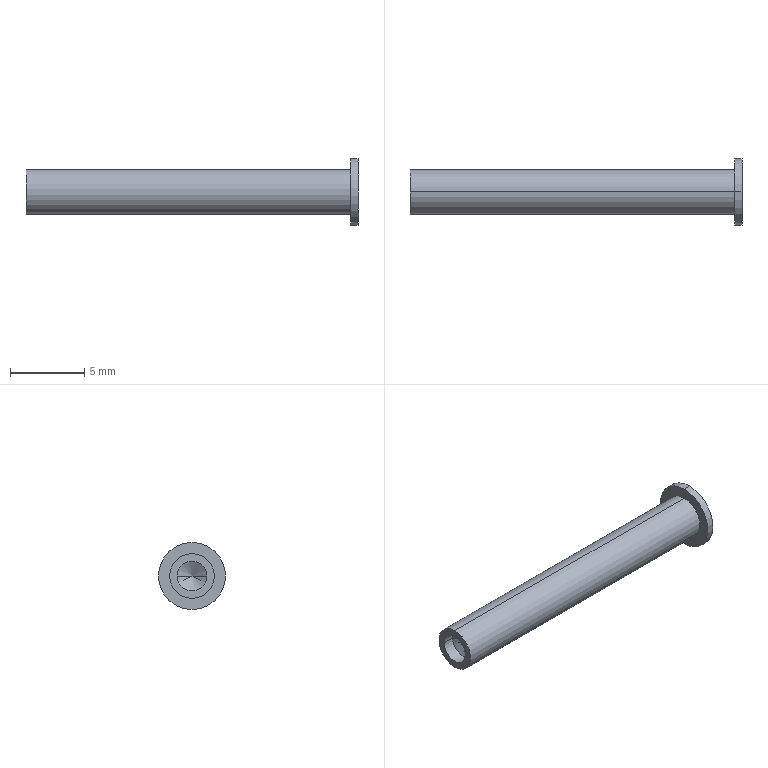Part | STEP file | _X2_751F4E45_X0_MS731-1_X2_8_11 | 1 solid | 11 faces | box 22.3 x 4.5 x 4.5 mm | volume 158.929 mm3 | cylinder 6 | plane 3 | cone 2 | commonest cylinder face diameters 2 x2 3 x2 4.5 x2
STEP:
#1=CARTESIAN_POINT('',(0.,0.,0.));
#2=DIRECTION('',(0.,0.,1.));
#3=DIRECTION('',(1.,0.,0.));
#4=AXIS2_PLACEMENT_3D('',#1,#2,#3);
#5=CARTESIAN_POINT('',(26.2,21.281,-110.75));
#6=VERTEX_POINT('',#5);
#7=CARTESIAN_POINT('',(26.2,21.281,-106.25));
#8=VERTEX_POINT('',#7);
#9=CARTESIAN_POINT('',(26.2,21.281,-108.5));
#10=DIRECTION('',(-1.,0.,0.));
#11=DIRECTION('',(0.,0.,-1.));
#12=AXIS2_PLACEMENT_3D('',#9,#10,#11);
#13=CIRCLE('',#12,2.25);
#14=CARTESIAN_POINT('',(26.2,21.281,-108.5));
#15=DIRECTION('',(-1.,0.,0.));
#16=DIRECTION('',(0.,0.,1.));
#17=AXIS2_PLACEMENT_3D('',#14,#15,#16);
#18=PLANE('',#17);
#19=CARTESIAN_POINT('',(0.,0.));
#20=DIRECTION('',(-1.,0.));
#21=AXIS2_PLACEMENT_2D('',#19,#20);
#22=CIRCLE('',#21,2.25);
#23=(GEOMETRIC_REPRESENTATION_CONTEXT(2)PARAMETRIC_REPRESENTATION_CONTEXT()REPRESENTATION_CONTEXT('',''));
#24=DEFINITIONAL_REPRESENTATION('',(#22),#23);
#25=PCURVE('',#18,#24);
#26=CARTESIAN_POINT('',(27.815,21.281,-108.5));
#27=DIRECTION('',(-1.,0.,0.));
#28=DIRECTION('',(0.,0.,1.));
#29=AXIS2_PLACEMENT_3D('',#26,#27,#28);
#30=CYLINDRICAL_SURFACE('',#29,2.25);
#31=CARTESIAN_POINT('',(3.142,1.615));
#32=DIRECTION('',(1.,0.));
#33=VECTOR('',#32,1.);
#34=LINE('',#31,#33);
#35=(GEOMETRIC_REPRESENTATION_CONTEXT(2)PARAMETRIC_REPRESENTATION_CONTEXT()REPRESENTATION_CONTEXT('',''));
#36=DEFINITIONAL_REPRESENTATION('',(#34),#35);
#37=PCURVE('',#30,#36);
#38=SURFACE_CURVE('',#13,(#25,#37),.PCURVE_S1.);
#39=EDGE_CURVE('',#6,#8,#38,.T.);
#40=ORIENTED_EDGE('',*,*,#39,.F.);
#41=CARTESIAN_POINT('',(26.2,21.281,-108.5));
#42=DIRECTION('',(-1.,0.,0.));
#43=DIRECTION('',(0.,0.,1.));
#44=AXIS2_PLACEMENT_3D('',#41,#42,#43);
#45=CIRCLE('',#44,2.25);
#46=CARTESIAN_POINT('',(0.,0.));
#47=DIRECTION('',(1.,0.));
#48=AXIS2_PLACEMENT_2D('',#46,#47);
#49=CIRCLE('',#48,2.25);
#50=(GEOMETRIC_REPRESENTATION_CONTEXT(2)PARAMETRIC_REPRESENTATION_CONTEXT()REPRESENTATION_CONTEXT('',''));
#51=DEFINITIONAL_REPRESENTATION('',(#49),#50);
#52=PCURVE('',#18,#51);
#53=CARTESIAN_POINT('',(27.815,21.281,-108.5));
#54=DIRECTION('',(-1.,0.,0.));
#55=DIRECTION('',(0.,0.,1.));
#56=AXIS2_PLACEMENT_3D('',#53,#54,#55);
#57=CYLINDRICAL_SURFACE('',#56,2.25);
#58=CARTESIAN_POINT('',(0.,1.615));
#59=DIRECTION('',(1.,0.));
#60=VECTOR('',#59,1.);
#61=LINE('',#58,#60);
#62=(GEOMETRIC_REPRESENTATION_CONTEXT(2)PARAMETRIC_REPRESENTATION_CONTEXT()REPRESENTATION_CONTEXT('',''));
#63=DEFINITIONAL_REPRESENTATION('',(#61),#62);
#64=PCURVE('',#57,#63);
#65=SURFACE_CURVE('',#45,(#52,#64),.PCURVE_S1.);
#66=EDGE_CURVE('',#8,#6,#65,.T.);
#67=ORIENTED_EDGE('',*,*,#66,.F.);
#68=EDGE_LOOP('',(#40,#67));
#69=FACE_BOUND('',#68,.F.);
#70=CARTESIAN_POINT('',(26.2,21.281,-110.));
#71=VERTEX_POINT('',#70);
#72=CARTESIAN_POINT('',(26.2,21.281,-107.));
#73=VERTEX_POINT('',#72);
#74=CARTESIAN_POINT('',(26.2,21.281,-108.5));
#75=DIRECTION('',(1.,0.,0.));
#76=DIRECTION('',(0.,0.,-1.));
#77=AXIS2_PLACEMENT_3D('',#74,#75,#76);
#78=CIRCLE('',#77,1.5);
#79=CARTESIAN_POINT('',(-1.5,0.));
#80=CARTESIAN_POINT('',(-1.5,2.598));
#81=CARTESIAN_POINT('',(0.75,1.299));
#82=CARTESIAN_POINT('',(3.,0.));
#83=CARTESIAN_POINT('',(0.75,-1.299));
#84=CARTESIAN_POINT('',(-1.5,-2.598));
#85=CARTESIAN_POINT('',(-1.5,0.));
#86=(BOUNDED_CURVE()B_SPLINE_CURVE(2,(#79,#80,#81,#82,#83,#84,#85),.UNSPECIFIED.,.T.,.F.)B_SPLINE_CURVE_WITH_KNOTS((1,2,2,2,2,1),(-2.094,0.,2.094,4.189,6.283,8.378),.UNSPECIFIED.)CURVE()GEOMETRIC_REPRESENTATION_ITEM()RATIONAL_B_SPLINE_CURVE((1.,0.5,1.,0.5,1.,0.5,1.))REPRESENTATION_ITEM(''));
#87=(GEOMETRIC_REPRESENTATION_CONTEXT(2)PARAMETRIC_REPRESENTATION_CONTEXT()REPRESENTATION_CONTEXT('',''));
#88=DEFINITIONAL_REPRESENTATION('',(#86),#87);
#89=PCURVE('',#18,#88);
#90=CARTESIAN_POINT('',(27.815,21.281,-108.5));
#91=DIRECTION('',(-1.,0.,0.));
#92=DIRECTION('',(0.,0.,1.));
#93=AXIS2_PLACEMENT_3D('',#90,#91,#92);
#94=CYLINDRICAL_SURFACE('',#93,1.5);
#95=CARTESIAN_POINT('',(3.142,1.615));
#96=DIRECTION('',(-1.,0.));
#97=VECTOR('',#96,1.);
#98=LINE('',#95,#97);
#99=(GEOMETRIC_REPRESENTATION_CONTEXT(2)PARAMETRIC_REPRESENTATION_CONTEXT()REPRESENTATION_CONTEXT('',''));
#100=DEFINITIONAL_REPRESENTATION('',(#98),#99);
#101=PCURVE('',#94,#100);
#102=SURFACE_CURVE('',#78,(#89,#101),.PCURVE_S1.);
#103=EDGE_CURVE('',#71,#73,#102,.T.);
#104=ORIENTED_EDGE('',*,*,#103,.F.);
#105=CARTESIAN_POINT('',(26.2,21.281,-108.5));
#106=DIRECTION('',(1.,0.,0.));
#107=DIRECTION('',(0.,0.,1.));
#108=AXIS2_PLACEMENT_3D('',#105,#106,#107);
#109=CIRCLE('',#108,1.5);
#110=CARTESIAN_POINT('',(1.5,0.));
#111=CARTESIAN_POINT('',(1.5,-2.598));
#112=CARTESIAN_POINT('',(-0.75,-1.299));
#113=CARTESIAN_POINT('',(-3.,0.));
#114=CARTESIAN_POINT('',(-0.75,1.299));
#115=CARTESIAN_POINT('',(1.5,2.598));
#116=CARTESIAN_POINT('',(1.5,0.));
#117=(BOUNDED_CURVE()B_SPLINE_CURVE(2,(#110,#111,#112,#113,#114,#115,#116),.UNSPECIFIED.,.T.,.F.)B_SPLINE_CURVE_WITH_KNOTS((1,2,2,2,2,1),(-2.094,0.,2.094,4.189,6.283,8.378),.UNSPECIFIED.)CURVE()GEOMETRIC_REPRESENTATION_ITEM()RATIONAL_B_SPLINE_CURVE((1.,0.5,1.,0.5,1.,0.5,1.))REPRESENTATION_ITEM(''));
#118=(GEOMETRIC_REPRESENTATION_CONTEXT(2)PARAMETRIC_REPRESENTATION_CONTEXT()REPRESENTATION_CONTEXT('',''));
#119=DEFINITIONAL_REPRESENTATION('',(#117),#118);
#120=PCURVE('',#18,#119);
#121=CARTESIAN_POINT('',(27.815,21.281,-108.5));
#122=DIRECTION('',(-1.,0.,0.));
#123=DIRECTION('',(0.,0.,1.));
#124=AXIS2_PLACEMENT_3D('',#121,#122,#123);
#125=CYLINDRICAL_SURFACE('',#124,1.5);
#126=CARTESIAN_POINT('',(6.283,1.615));
#127=DIRECTION('',(-1.,0.));
#128=VECTOR('',#127,1.);
#129=LINE('',#126,#128);
#130=(GEOMETRIC_REPRESENTATION_CONTEXT(2)PARAMETRIC_REPRESENTATION_CONTEXT()REPRESENTATION_CONTEXT('',''));
#131=DEFINITIONAL_REPRESENTATION('',(#129),#130);
#132=PCURVE('',#125,#131);
#133=SURFACE_CURVE('',#109,(#120,#132),.PCURVE_S1.);
#134=EDGE_CURVE('',#73,#71,#133,.T.);
#135=ORIENTED_EDGE('',*,*,#134,.F.);
#136=EDGE_LOOP('',(#104,#135));
#137=FACE_BOUND('',#136,.F.);
#138=ADVANCED_FACE('',(#69,#137),#18,.T.);
#139=CARTESIAN_POINT('',(26.7,21.281,-110.75));
#140=VERTEX_POINT('',#139);
#141=CARTESIAN_POINT('',(26.2,21.281,-110.75));
#142=DIRECTION('',(1.,0.,0.));
#143=VECTOR('',#142,1.);
#144=LINE('',#141,#143);
#145=CARTESIAN_POINT('',(3.142,1.615));
#146=DIRECTION('',(0.,-1.));
#147=VECTOR('',#146,1.);
#148=LINE('',#145,#147);
#149=(GEOMETRIC_REPRESENTATION_CONTEXT(2)PARAMETRIC_REPRESENTATION_CONTEXT()REPRESENTATION_CONTEXT('',''));
#150=DEFINITIONAL_REPRESENTATION('',(#148),#149);
#151=PCURVE('',#30,#150);
#152=CARTESIAN_POINT('',(3.142,1.615));
#153=DIRECTION('',(0.,-1.));
#154=VECTOR('',#153,1.);
#155=LINE('',#152,#154);
#156=(GEOMETRIC_REPRESENTATION_CONTEXT(2)PARAMETRIC_REPRESENTATION_CONTEXT()REPRESENTATION_CONTEXT('',''));
#157=DEFINITIONAL_REPRESENTATION('',(#155),#156);
#158=PCURVE('',#57,#157);
#159=SURFACE_CURVE('',#144,(#151,#158),.PCURVE_S1.);
#160=EDGE_CURVE('',#6,#140,#159,.T.);
#161=ORIENTED_EDGE('',*,*,#160,.T.);
#162=CARTESIAN_POINT('',(26.7,21.281,-106.25));
#163=VERTEX_POINT('',#162);
#164=CARTESIAN_POINT('',(26.7,21.281,-108.5));
#165=DIRECTION('',(1.,0.,0.));
#166=DIRECTION('',(0.,0.,1.));
#167=AXIS2_PLACEMENT_3D('',#164,#165,#166);
#168=CIRCLE('',#167,2.25);
#169=CARTESIAN_POINT('',(6.283,1.115));
#170=DIRECTION('',(-1.,0.));
#171=VECTOR('',#170,1.);
#172=LINE('',#169,#171);
#173=(GEOMETRIC_REPRESENTATION_CONTEXT(2)PARAMETRIC_REPRESENTATION_CONTEXT()REPRESENTATION_CONTEXT('',''));
#174=DEFINITIONAL_REPRESENTATION('',(#172),#173);
#175=PCURVE('',#30,#174);
#176=CARTESIAN_POINT('',(26.7,21.281,-108.5));
#177=DIRECTION('',(-1.,0.,0.));
#178=DIRECTION('',(0.,0.,1.));
#179=AXIS2_PLACEMENT_3D('',#176,#177,#178);
#180=PLANE('',#179);
#181=CARTESIAN_POINT('',(2.25,0.));
#182=CARTESIAN_POINT('',(2.25,-3.897));
#183=CARTESIAN_POINT('',(-1.125,-1.949));
#184=CARTESIAN_POINT('',(-4.5,0.));
#185=CARTESIAN_POINT('',(-1.125,1.949));
#186=CARTESIAN_POINT('',(2.25,3.897));
#187=CARTESIAN_POINT('',(2.25,0.));
#188=(BOUNDED_CURVE()B_SPLINE_CURVE(2,(#181,#182,#183,#184,#185,#186,#187),.UNSPECIFIED.,.T.,.F.)B_SPLINE_CURVE_WITH_KNOTS((1,2,2,2,2,1),(-2.094,0.,2.094,4.189,6.283,8.378),.UNSPECIFIED.)CURVE()GEOMETRIC_REPRESENTATION_ITEM()RATIONAL_B_SPLINE_CURVE((1.,0.5,1.,0.5,1.,0.5,1.))REPRESENTATION_ITEM(''));
#189=(GEOMETRIC_REPRESENTATION_CONTEXT(2)PARAMETRIC_REPRESENTATION_CONTEXT()REPRESENTATION_CONTEXT('',''));
#190=DEFINITIONAL_REPRESENTATION('',(#188),#189);
#191=PCURVE('',#180,#190);
#192=SURFACE_CURVE('',#168,(#175,#191),.PCURVE_S1.);
#193=EDGE_CURVE('',#163,#140,#192,.T.);
#194=ORIENTED_EDGE('',*,*,#193,.F.);
#195=CARTESIAN_POINT('',(26.2,21.281,-106.25));
#196=DIRECTION('',(1.,0.,0.));
#197=VECTOR('',#196,1.);
#198=LINE('',#195,#197);
#199=CARTESIAN_POINT('',(6.283,1.615));
#200=DIRECTION('',(0.,-1.));
#201=VECTOR('',#200,1.);
#202=LINE('',#199,#201);
#203=(GEOMETRIC_REPRESENTATION_CONTEXT(2)PARAMETRIC_REPRESENTATION_CONTEXT()REPRESENTATION_CONTEXT('',''));
#204=DEFINITIONAL_REPRESENTATION('',(#202),#203);
#205=PCURVE('',#30,#204);
#206=CARTESIAN_POINT('',(0.,1.615));
#207=DIRECTION('',(0.,-1.));
#208=VECTOR('',#207,1.);
#209=LINE('',#206,#208);
#210=(GEOMETRIC_REPRESENTATION_CONTEXT(2)PARAMETRIC_REPRESENTATION_CONTEXT()REPRESENTATION_CONTEXT('',''));
#211=DEFINITIONAL_REPRESENTATION('',(#209),#210);
#212=PCURVE('',#57,#211);
#213=SURFACE_CURVE('',#198,(#205,#212),.PCURVE_S1.);
#214=EDGE_CURVE('',#8,#163,#213,.T.);
#215=ORIENTED_EDGE('',*,*,#214,.F.);
#216=ORIENTED_EDGE('',*,*,#39,.F.);
#217=EDGE_LOOP('',(#161,#194,#215,#216));
#218=FACE_BOUND('',#217,.T.);
#219=ADVANCED_FACE('',(#218),#30,.T.);
#220=ORIENTED_EDGE('',*,*,#160,.F.);
#221=ORIENTED_EDGE('',*,*,#66,.F.);
#222=ORIENTED_EDGE('',*,*,#214,.T.);
#223=CARTESIAN_POINT('',(26.7,21.281,-108.5));
#224=DIRECTION('',(1.,0.,0.));
#225=DIRECTION('',(0.,0.,-1.));
#226=AXIS2_PLACEMENT_3D('',#223,#224,#225);
#227=CIRCLE('',#226,2.25);
#228=CARTESIAN_POINT('',(3.142,1.115));
#229=DIRECTION('',(-1.,0.));
#230=VECTOR('',#229,1.);
#231=LINE('',#228,#230);
#232=(GEOMETRIC_REPRESENTATION_CONTEXT(2)PARAMETRIC_REPRESENTATION_CONTEXT()REPRESENTATION_CONTEXT('',''));
#233=DEFINITIONAL_REPRESENTATION('',(#231),#232);
#234=PCURVE('',#57,#233);
#235=CARTESIAN_POINT('',(-2.25,0.));
#236=CARTESIAN_POINT('',(-2.25,3.897));
#237=CARTESIAN_POINT('',(1.125,1.949));
#238=CARTESIAN_POINT('',(4.5,0.));
#239=CARTESIAN_POINT('',(1.125,-1.949));
#240=CARTESIAN_POINT('',(-2.25,-3.897));
#241=CARTESIAN_POINT('',(-2.25,0.));
#242=(BOUNDED_CURVE()B_SPLINE_CURVE(2,(#235,#236,#237,#238,#239,#240,#241),.UNSPECIFIED.,.T.,.F.)B_SPLINE_CURVE_WITH_KNOTS((1,2,2,2,2,1),(-2.094,0.,2.094,4.189,6.283,8.378),.UNSPECIFIED.)CURVE()GEOMETRIC_REPRESENTATION_ITEM()RATIONAL_B_SPLINE_CURVE((1.,0.5,1.,0.5,1.,0.5,1.))REPRESENTATION_ITEM(''));
#243=(GEOMETRIC_REPRESENTATION_CONTEXT(2)PARAMETRIC_REPRESENTATION_CONTEXT()REPRESENTATION_CONTEXT('',''));
#244=DEFINITIONAL_REPRESENTATION('',(#242),#243);
#245=PCURVE('',#180,#244);
#246=SURFACE_CURVE('',#227,(#234,#245),.PCURVE_S1.);
#247=EDGE_CURVE('',#140,#163,#246,.T.);
#248=ORIENTED_EDGE('',*,*,#247,.F.);
#249=EDGE_LOOP('',(#220,#221,#222,#248));
#250=FACE_BOUND('',#249,.T.);
#251=ADVANCED_FACE('',(#250),#57,.T.);
#252=ORIENTED_EDGE('',*,*,#247,.F.);
#253=ORIENTED_EDGE('',*,*,#193,.F.);
#254=EDGE_LOOP('',(#252,#253));
#255=FACE_BOUND('',#254,.F.);
#256=ADVANCED_FACE('',(#255),#180,.F.);
#257=CARTESIAN_POINT('',(4.4,21.281,-110.));
#258=VERTEX_POINT('',#257);
#259=CARTESIAN_POINT('',(4.4,21.281,-110.));
#260=DIRECTION('',(1.,0.,0.));
#261=VECTOR('',#260,1.);
#262=LINE('',#259,#261);
#263=CARTESIAN_POINT('',(3.142,23.415));
#264=DIRECTION('',(0.,-1.));
#265=VECTOR('',#264,1.);
#266=LINE('',#263,#265);
#267=(GEOMETRIC_REPRESENTATION_CONTEXT(2)PARAMETRIC_REPRESENTATION_CONTEXT()REPRESENTATION_CONTEXT('',''));
#268=DEFINITIONAL_REPRESENTATION('',(#266),#267);
#269=PCURVE('',#94,#268);
#270=CARTESIAN_POINT('',(3.142,23.415));
#271=DIRECTION('',(0.,-1.));
#272=VECTOR('',#271,1.);
#273=LINE('',#270,#272);
#274=(GEOMETRIC_REPRESENTATION_CONTEXT(2)PARAMETRIC_REPRESENTATION_CONTEXT()REPRESENTATION_CONTEXT('',''));
#275=DEFINITIONAL_REPRESENTATION('',(#273),#274);
#276=PCURVE('',#125,#275);
#277=SURFACE_CURVE('',#262,(#269,#276),.PCURVE_S1.);
#278=EDGE_CURVE('',#258,#71,#277,.T.);
#279=ORIENTED_EDGE('',*,*,#278,.F.);
#280=CARTESIAN_POINT('',(4.4,21.281,-107.));
#281=VERTEX_POINT('',#280);
#282=CARTESIAN_POINT('',(4.4,21.281,-108.5));
#283=DIRECTION('',(-1.,0.,0.));
#284=DIRECTION('',(0.,0.,1.));
#285=AXIS2_PLACEMENT_3D('',#282,#283,#284);
#286=CIRCLE('',#285,1.5);
#287=CARTESIAN_POINT('',(0.,23.415));
#288=DIRECTION('',(1.,0.));
#289=VECTOR('',#288,1.);
#290=LINE('',#287,#289);
#291=(GEOMETRIC_REPRESENTATION_CONTEXT(2)PARAMETRIC_REPRESENTATION_CONTEXT()REPRESENTATION_CONTEXT('',''));
#292=DEFINITIONAL_REPRESENTATION('',(#290),#291);
#293=PCURVE('',#94,#292);
#294=CARTESIAN_POINT('',(4.4,21.281,-108.5));
#295=DIRECTION('',(-1.,0.,0.));
#296=DIRECTION('',(0.,0.,1.));
#297=AXIS2_PLACEMENT_3D('',#294,#295,#296);
#298=PLANE('',#297);
#299=CARTESIAN_POINT('',(0.,0.));
#300=DIRECTION('',(1.,0.));
#301=AXIS2_PLACEMENT_2D('',#299,#300);
#302=CIRCLE('',#301,1.5);
#303=(GEOMETRIC_REPRESENTATION_CONTEXT(2)PARAMETRIC_REPRESENTATION_CONTEXT()REPRESENTATION_CONTEXT('',''));
#304=DEFINITIONAL_REPRESENTATION('',(#302),#303);
#305=PCURVE('',#298,#304);
#306=SURFACE_CURVE('',#286,(#293,#305),.PCURVE_S1.);
#307=EDGE_CURVE('',#281,#258,#306,.T.);
#308=ORIENTED_EDGE('',*,*,#307,.F.);
#309=CARTESIAN_POINT('',(4.4,21.281,-107.));
#310=DIRECTION('',(1.,0.,0.));
#311=VECTOR('',#310,1.);
#312=LINE('',#309,#311);
#313=CARTESIAN_POINT('',(0.,23.415));
#314=DIRECTION('',(0.,-1.));
#315=VECTOR('',#314,1.);
#316=LINE('',#313,#315);
#317=(GEOMETRIC_REPRESENTATION_CONTEXT(2)PARAMETRIC_REPRESENTATION_CONTEXT()REPRESENTATION_CONTEXT('',''));
#318=DEFINITIONAL_REPRESENTATION('',(#316),#317);
#319=PCURVE('',#94,#318);
#320=CARTESIAN_POINT('',(6.283,23.415));
#321=DIRECTION('',(0.,-1.));
#322=VECTOR('',#321,1.);
#323=LINE('',#320,#322);
#324=(GEOMETRIC_REPRESENTATION_CONTEXT(2)PARAMETRIC_REPRESENTATION_CONTEXT()REPRESENTATION_CONTEXT('',''));
#325=DEFINITIONAL_REPRESENTATION('',(#323),#324);
#326=PCURVE('',#125,#325);
#327=SURFACE_CURVE('',#312,(#319,#326),.PCURVE_S1.);
#328=EDGE_CURVE('',#281,#73,#327,.T.);
#329=ORIENTED_EDGE('',*,*,#328,.T.);
#330=ORIENTED_EDGE('',*,*,#103,.F.);
#331=EDGE_LOOP('',(#279,#308,#329,#330));
#332=FACE_BOUND('',#331,.T.);
#333=ADVANCED_FACE('',(#332),#94,.T.);
#334=ORIENTED_EDGE('',*,*,#278,.T.);
#335=ORIENTED_EDGE('',*,*,#134,.F.);
#336=ORIENTED_EDGE('',*,*,#328,.F.);
#337=CARTESIAN_POINT('',(4.4,21.281,-108.5));
#338=DIRECTION('',(-1.,0.,0.));
#339=DIRECTION('',(0.,0.,-1.));
#340=AXIS2_PLACEMENT_3D('',#337,#338,#339);
#341=CIRCLE('',#340,1.5);
#342=CARTESIAN_POINT('',(3.142,23.415));
#343=DIRECTION('',(1.,0.));
#344=VECTOR('',#343,1.);
#345=LINE('',#342,#344);
#346=(GEOMETRIC_REPRESENTATION_CONTEXT(2)PARAMETRIC_REPRESENTATION_CONTEXT()REPRESENTATION_CONTEXT('',''));
#347=DEFINITIONAL_REPRESENTATION('',(#345),#346);
#348=PCURVE('',#125,#347);
#349=CARTESIAN_POINT('',(0.,0.));
#350=DIRECTION('',(-1.,0.));
#351=AXIS2_PLACEMENT_2D('',#349,#350);
#352=CIRCLE('',#351,1.5);
#353=(GEOMETRIC_REPRESENTATION_CONTEXT(2)PARAMETRIC_REPRESENTATION_CONTEXT()REPRESENTATION_CONTEXT('',''));
#354=DEFINITIONAL_REPRESENTATION('',(#352),#353);
#355=PCURVE('',#298,#354);
#356=SURFACE_CURVE('',#341,(#348,#355),.PCURVE_S1.);
#357=EDGE_CURVE('',#258,#281,#356,.T.);
#358=ORIENTED_EDGE('',*,*,#357,.F.);
#359=EDGE_LOOP('',(#334,#335,#336,#358));
#360=FACE_BOUND('',#359,.T.);
#361=ADVANCED_FACE('',(#360),#125,.T.);
#362=ORIENTED_EDGE('',*,*,#307,.F.);
#363=ORIENTED_EDGE('',*,*,#357,.F.);
#364=EDGE_LOOP('',(#362,#363));
#365=FACE_BOUND('',#364,.F.);
#366=CARTESIAN_POINT('',(4.4,22.281,-108.5));
#367=VERTEX_POINT('',#366);
#368=CARTESIAN_POINT('',(4.4,20.281,-108.5));
#369=VERTEX_POINT('',#368);
#370=CARTESIAN_POINT('',(4.4,21.281,-108.5));
#371=DIRECTION('',(1.,0.,0.));
#372=DIRECTION('',(0.,1.,0.));
#373=AXIS2_PLACEMENT_3D('',#370,#371,#372);
#374=CIRCLE('',#373,1.);
#375=CARTESIAN_POINT('',(0.,1.));
#376=CARTESIAN_POINT('',(1.732,1.));
#377=CARTESIAN_POINT('',(0.866,-0.5));
#378=CARTESIAN_POINT('',(0.,-2.));
#379=CARTESIAN_POINT('',(-0.866,-0.5));
#380=CARTESIAN_POINT('',(-1.732,1.));
#381=CARTESIAN_POINT('',(0.,1.));
#382=(BOUNDED_CURVE()B_SPLINE_CURVE(2,(#375,#376,#377,#378,#379,#380,#381),.UNSPECIFIED.,.T.,.F.)B_SPLINE_CURVE_WITH_KNOTS((1,2,2,2,2,1),(-2.094,0.,2.094,4.189,6.283,8.378),.UNSPECIFIED.)CURVE()GEOMETRIC_REPRESENTATION_ITEM()RATIONAL_B_SPLINE_CURVE((1.,0.5,1.,0.5,1.,0.5,1.))REPRESENTATION_ITEM(''));
#383=(GEOMETRIC_REPRESENTATION_CONTEXT(2)PARAMETRIC_REPRESENTATION_CONTEXT()REPRESENTATION_CONTEXT('',''));
#384=DEFINITIONAL_REPRESENTATION('',(#382),#383);
#385=PCURVE('',#298,#384);
#386=CARTESIAN_POINT('',(4.331,21.281,-108.5));
#387=DIRECTION('',(1.,0.,0.));
#388=DIRECTION('',(0.,1.,0.));
#389=AXIS2_PLACEMENT_3D('',#386,#387,#388);
#390=CYLINDRICAL_SURFACE('',#389,1.);
#391=CARTESIAN_POINT('',(0.,0.06887));
#392=DIRECTION('',(1.,0.));
#393=VECTOR('',#392,1.);
#394=LINE('',#391,#393);
#395=(GEOMETRIC_REPRESENTATION_CONTEXT(2)PARAMETRIC_REPRESENTATION_CONTEXT()REPRESENTATION_CONTEXT('',''));
#396=DEFINITIONAL_REPRESENTATION('',(#394),#395);
#397=PCURVE('',#390,#396);
#398=SURFACE_CURVE('',#374,(#385,#397),.PCURVE_S1.);
#399=EDGE_CURVE('',#367,#369,#398,.T.);
#400=ORIENTED_EDGE('',*,*,#399,.F.);
#401=CARTESIAN_POINT('',(4.4,21.281,-108.5));
#402=DIRECTION('',(1.,0.,0.));
#403=DIRECTION('',(0.,-1.,0.));
#404=AXIS2_PLACEMENT_3D('',#401,#402,#403);
#405=CIRCLE('',#404,1.);
#406=CARTESIAN_POINT('',(0.,-1.));
#407=CARTESIAN_POINT('',(-1.732,-1.));
#408=CARTESIAN_POINT('',(-0.866,0.5));
#409=CARTESIAN_POINT('',(0.,2.));
#410=CARTESIAN_POINT('',(0.866,0.5));
#411=CARTESIAN_POINT('',(1.732,-1.));
#412=CARTESIAN_POINT('',(0.,-1.));
#413=(BOUNDED_CURVE()B_SPLINE_CURVE(2,(#406,#407,#408,#409,#410,#411,#412),.UNSPECIFIED.,.T.,.F.)B_SPLINE_CURVE_WITH_KNOTS((1,2,2,2,2,1),(-2.094,0.,2.094,4.189,6.283,8.378),.UNSPECIFIED.)CURVE()GEOMETRIC_REPRESENTATION_ITEM()RATIONAL_B_SPLINE_CURVE((1.,0.5,1.,0.5,1.,0.5,1.))REPRESENTATION_ITEM(''));
#414=(GEOMETRIC_REPRESENTATION_CONTEXT(2)PARAMETRIC_REPRESENTATION_CONTEXT()REPRESENTATION_CONTEXT('',''));
#415=DEFINITIONAL_REPRESENTATION('',(#413),#414);
#416=PCURVE('',#298,#415);
#417=CARTESIAN_POINT('',(4.331,21.281,-108.5));
#418=DIRECTION('',(1.,0.,0.));
#419=DIRECTION('',(0.,1.,0.));
#420=AXIS2_PLACEMENT_3D('',#417,#418,#419);
#421=CYLINDRICAL_SURFACE('',#420,1.);
#422=CARTESIAN_POINT('',(3.142,0.06887));
#423=DIRECTION('',(1.,0.));
#424=VECTOR('',#423,1.);
#425=LINE('',#422,#424);
#426=(GEOMETRIC_REPRESENTATION_CONTEXT(2)PARAMETRIC_REPRESENTATION_CONTEXT()REPRESENTATION_CONTEXT('',''));
#427=DEFINITIONAL_REPRESENTATION('',(#425),#426);
#428=PCURVE('',#421,#427);
#429=SURFACE_CURVE('',#405,(#416,#428),.PCURVE_S1.);
#430=EDGE_CURVE('',#369,#367,#429,.T.);
#431=ORIENTED_EDGE('',*,*,#430,.F.);
#432=EDGE_LOOP('',(#400,#431));
#433=FACE_BOUND('',#432,.F.);
#434=ADVANCED_FACE('',(#365,#433),#298,.T.);
#435=CARTESIAN_POINT('',(4.7,22.281,-108.5));
#436=VERTEX_POINT('',#435);
#437=CARTESIAN_POINT('',(4.4,22.281,-108.5));
#438=DIRECTION('',(1.,0.,0.));
#439=VECTOR('',#438,1.);
#440=LINE('',#437,#439);
#441=CARTESIAN_POINT('',(0.,0.06887));
#442=DIRECTION('',(0.,1.));
#443=VECTOR('',#442,1.);
#444=LINE('',#441,#443);
#445=(GEOMETRIC_REPRESENTATION_CONTEXT(2)PARAMETRIC_REPRESENTATION_CONTEXT()REPRESENTATION_CONTEXT('',''));
#446=DEFINITIONAL_REPRESENTATION('',(#444),#445);
#447=PCURVE('',#390,#446);
#448=CARTESIAN_POINT('',(6.283,0.06887));
#449=DIRECTION('',(0.,1.));
#450=VECTOR('',#449,1.);
#451=LINE('',#448,#450);
#452=(GEOMETRIC_REPRESENTATION_CONTEXT(2)PARAMETRIC_REPRESENTATION_CONTEXT()REPRESENTATION_CONTEXT('',''));
#453=DEFINITIONAL_REPRESENTATION('',(#451),#452);
#454=PCURVE('',#421,#453);
#455=SURFACE_CURVE('',#440,(#447,#454),.PCURVE_S1.);
#456=EDGE_CURVE('',#367,#436,#455,.T.);
#457=ORIENTED_EDGE('',*,*,#456,.F.);
#458=ORIENTED_EDGE('',*,*,#399,.T.);
#459=CARTESIAN_POINT('',(4.7,20.281,-108.5));
#460=VERTEX_POINT('',#459);
#461=CARTESIAN_POINT('',(4.4,20.281,-108.5));
#462=DIRECTION('',(1.,0.,0.));
#463=VECTOR('',#462,1.);
#464=LINE('',#461,#463);
#465=CARTESIAN_POINT('',(3.142,0.06887));
#466=DIRECTION('',(0.,1.));
#467=VECTOR('',#466,1.);
#468=LINE('',#465,#467);
#469=(GEOMETRIC_REPRESENTATION_CONTEXT(2)PARAMETRIC_REPRESENTATION_CONTEXT()REPRESENTATION_CONTEXT('',''));
#470=DEFINITIONAL_REPRESENTATION('',(#468),#469);
#471=PCURVE('',#390,#470);
#472=CARTESIAN_POINT('',(3.142,0.06887));
#473=DIRECTION('',(0.,1.));
#474=VECTOR('',#473,1.);
#475=LINE('',#472,#474);
#476=(GEOMETRIC_REPRESENTATION_CONTEXT(2)PARAMETRIC_REPRESENTATION_CONTEXT()REPRESENTATION_CONTEXT('',''));
#477=DEFINITIONAL_REPRESENTATION('',(#475),#476);
#478=PCURVE('',#421,#477);
#479=SURFACE_CURVE('',#464,(#471,#478),.PCURVE_S1.);
#480=EDGE_CURVE('',#369,#460,#479,.T.);
#481=ORIENTED_EDGE('',*,*,#480,.T.);
#482=CARTESIAN_POINT('',(5.2,20.281,-108.5));
#483=VERTEX_POINT('',#482);
#484=CARTESIAN_POINT('',(4.7,20.281,-108.5));
#485=DIRECTION('',(1.,0.,0.));
#486=VECTOR('',#485,1.);
#487=LINE('',#484,#486);
#488=CARTESIAN_POINT('',(3.142,0.3689));
#489=DIRECTION('',(0.,1.));
#490=VECTOR('',#489,1.);
#491=LINE('',#488,#490);
#492=(GEOMETRIC_REPRESENTATION_CONTEXT(2)PARAMETRIC_REPRESENTATION_CONTEXT()REPRESENTATION_CONTEXT('',''));
#493=DEFINITIONAL_REPRESENTATION('',(#491),#492);
#494=PCURVE('',#390,#493);
#495=CARTESIAN_POINT('',(3.142,0.3689));
#496=DIRECTION('',(0.,1.));
#497=VECTOR('',#496,1.);
#498=LINE('',#495,#497);
#499=(GEOMETRIC_REPRESENTATION_CONTEXT(2)PARAMETRIC_REPRESENTATION_CONTEXT()REPRESENTATION_CONTEXT('',''));
#500=DEFINITIONAL_REPRESENTATION('',(#498),#499);
#501=PCURVE('',#421,#500);
#502=SURFACE_CURVE('',#487,(#494,#501),.PCURVE_S1.);
#503=EDGE_CURVE('',#460,#483,#502,.T.);
#504=ORIENTED_EDGE('',*,*,#503,.T.);
#505=CARTESIAN_POINT('',(5.2,22.281,-108.5));
#506=VERTEX_POINT('',#505);
#507=CARTESIAN_POINT('',(5.2,21.281,-108.5));
#508=DIRECTION('',(-1.,0.,0.));
#509=DIRECTION('',(0.,-1.,0.));
#510=AXIS2_PLACEMENT_3D('',#507,#508,#509);
#511=CIRCLE('',#510,1.);
#512=CARTESIAN_POINT('',(3.142,0.8689));
#513=DIRECTION('',(-1.,0.));
#514=VECTOR('',#513,1.);
#515=LINE('',#512,#514);
#516=(GEOMETRIC_REPRESENTATION_CONTEXT(2)PARAMETRIC_REPRESENTATION_CONTEXT()REPRESENTATION_CONTEXT('',''));
#517=DEFINITIONAL_REPRESENTATION('',(#515),#516);
#518=PCURVE('',#390,#517);
#519=CARTESIAN_POINT('',(5.482,21.281,-108.5));
#520=DIRECTION('',(-1.,0.,0.));
#521=DIRECTION('',(0.,-1.,0.));
#522=AXIS2_PLACEMENT_3D('',#519,#520,#521);
#523=CONICAL_SURFACE('',#522,0.5121,1.047);
#524=CARTESIAN_POINT('',(0.,0.2817));
#525=DIRECTION('',(1.,0.));
#526=VECTOR('',#525,1.);
#527=LINE('',#524,#526);
#528=(GEOMETRIC_REPRESENTATION_CONTEXT(2)PARAMETRIC_REPRESENTATION_CONTEXT()REPRESENTATION_CONTEXT('',''));
#529=DEFINITIONAL_REPRESENTATION('',(#527),#528);
#530=PCURVE('',#523,#529);
#531=SURFACE_CURVE('',#511,(#518,#530),.PCURVE_S1.);
#532=EDGE_CURVE('',#483,#506,#531,.T.);
#533=ORIENTED_EDGE('',*,*,#532,.T.);
#534=CARTESIAN_POINT('',(4.7,22.281,-108.5));
#535=DIRECTION('',(1.,0.,0.));
#536=VECTOR('',#535,1.);
#537=LINE('',#534,#536);
#538=CARTESIAN_POINT('',(0.,0.3689));
#539=DIRECTION('',(0.,1.));
#540=VECTOR('',#539,1.);
#541=LINE('',#538,#540);
#542=(GEOMETRIC_REPRESENTATION_CONTEXT(2)PARAMETRIC_REPRESENTATION_CONTEXT()REPRESENTATION_CONTEXT('',''));
#543=DEFINITIONAL_REPRESENTATION('',(#541),#542);
#544=PCURVE('',#390,#543);
#545=CARTESIAN_POINT('',(6.283,0.3689));
#546=DIRECTION('',(0.,1.));
#547=VECTOR('',#546,1.);
#548=LINE('',#545,#547);
#549=(GEOMETRIC_REPRESENTATION_CONTEXT(2)PARAMETRIC_REPRESENTATION_CONTEXT()REPRESENTATION_CONTEXT('',''));
#550=DEFINITIONAL_REPRESENTATION('',(#548),#549);
#551=PCURVE('',#421,#550);
#552=SURFACE_CURVE('',#537,(#544,#551),.PCURVE_S1.);
#553=EDGE_CURVE('',#436,#506,#552,.T.);
#554=ORIENTED_EDGE('',*,*,#553,.F.);
#555=EDGE_LOOP('',(#457,#458,#481,#504,#533,#554));
#556=FACE_BOUND('',#555,.F.);
#557=ADVANCED_FACE('',(#556),#390,.F.);
#558=ORIENTED_EDGE('',*,*,#480,.F.);
#559=ORIENTED_EDGE('',*,*,#430,.T.);
#560=ORIENTED_EDGE('',*,*,#456,.T.);
#561=ORIENTED_EDGE('',*,*,#553,.T.);
#562=CARTESIAN_POINT('',(5.2,21.281,-108.5));
#563=DIRECTION('',(-1.,0.,0.));
#564=DIRECTION('',(0.,1.,0.));
#565=AXIS2_PLACEMENT_3D('',#562,#563,#564);
#566=CIRCLE('',#565,1.);
#567=CARTESIAN_POINT('',(6.283,0.8689));
#568=DIRECTION('',(-1.,0.));
#569=VECTOR('',#568,1.);
#570=LINE('',#567,#569);
#571=(GEOMETRIC_REPRESENTATION_CONTEXT(2)PARAMETRIC_REPRESENTATION_CONTEXT()REPRESENTATION_CONTEXT('',''));
#572=DEFINITIONAL_REPRESENTATION('',(#570),#571);
#573=PCURVE('',#421,#572);
#574=CARTESIAN_POINT('',(5.482,21.281,-108.5));
#575=DIRECTION('',(-1.,0.,0.));
#576=DIRECTION('',(0.,-1.,0.));
#577=AXIS2_PLACEMENT_3D('',#574,#575,#576);
#578=CONICAL_SURFACE('',#577,0.5121,1.047);
#579=CARTESIAN_POINT('',(3.142,0.2817));
#580=DIRECTION('',(1.,0.));
#581=VECTOR('',#580,1.);
#582=LINE('',#579,#581);
#583=(GEOMETRIC_REPRESENTATION_CONTEXT(2)PARAMETRIC_REPRESENTATION_CONTEXT()REPRESENTATION_CONTEXT('',''));
#584=DEFINITIONAL_REPRESENTATION('',(#582),#583);
#585=PCURVE('',#578,#584);
#586=SURFACE_CURVE('',#566,(#573,#585),.PCURVE_S1.);
#587=EDGE_CURVE('',#506,#483,#586,.T.);
#588=ORIENTED_EDGE('',*,*,#587,.T.);
#589=ORIENTED_EDGE('',*,*,#503,.F.);
#590=EDGE_LOOP('',(#558,#559,#560,#561,#588,#589));
#591=FACE_BOUND('',#590,.F.);
#592=ADVANCED_FACE('',(#591),#421,.F.);
#593=CARTESIAN_POINT('',(5.777,21.281,-108.5));
#594=VERTEX_POINT('',#593);
#595=CARTESIAN_POINT('',(5.2,22.281,-108.5));
#596=DIRECTION('',(0.5,-0.866,0.));
#597=VECTOR('',#596,1.);
#598=LINE('',#595,#597);
#599=CARTESIAN_POINT('',(3.142,0.2817));
#600=CARTESIAN_POINT('',(3.142,0.273));
#601=CARTESIAN_POINT('',(3.142,0.2555));
#602=CARTESIAN_POINT('',(3.142,0.2292));
#603=CARTESIAN_POINT('',(3.142,0.203));
#604=CARTESIAN_POINT('',(3.142,0.1767));
#605=CARTESIAN_POINT('',(3.142,0.1505));
#606=CARTESIAN_POINT('',(3.142,0.1243));
#607=CARTESIAN_POINT('',(3.142,0.09802));
#608=CARTESIAN_POINT('',(3.142,0.07177));
#609=CARTESIAN_POINT('',(3.142,0.04553));
#610=CARTESIAN_POINT('',(3.142,0.01929));
#611=CARTESIAN_POINT('',(3.142,-0.006957));
#612=CARTESIAN_POINT('',(3.142,-0.0332));
#613=CARTESIAN_POINT('',(3.142,-0.05944));
#614=CARTESIAN_POINT('',(3.142,-0.08569));
#615=CARTESIAN_POINT('',(3.142,-0.1119));
#616=CARTESIAN_POINT('',(3.142,-0.1382));
#617=CARTESIAN_POINT('',(3.142,-0.1644));
#618=CARTESIAN_POINT('',(3.142,-0.1907));
#619=CARTESIAN_POINT('',(3.142,-0.2169));
#620=CARTESIAN_POINT('',(3.142,-0.2431));
#621=CARTESIAN_POINT('',(3.142,-0.2694));
#622=CARTESIAN_POINT('',(3.142,-0.2869));
#623=CARTESIAN_POINT('',(3.142,-0.2956));
#624=B_SPLINE_CURVE_WITH_KNOTS('',3,(#599,#600,#601,#602,#603,#604,#605,#606,#607,#608,#609,#610,#611,#612,#613,#614,#615,#616,#617,#618,#619,#620,#621,#622,#623),.UNSPECIFIED.,.F.,.F.,(4,1,1,1,1,1,1,1,1,1,1,1,1,1,1,1,1,1,1,1,1,1,4),(0.,0.05249,0.105,0.1575,0.2099,0.2624,0.3149,0.3674,0.4199,0.4724,0.5249,0.5774,0.6298,0.6823,0.7348,0.7873,0.8398,0.8923,0.9448,0.9972,1.05,1.102,1.155),.QUASI_UNIFORM_KNOTS.);
#625=(GEOMETRIC_REPRESENTATION_CONTEXT(2)PARAMETRIC_REPRESENTATION_CONTEXT()REPRESENTATION_CONTEXT('',''));
#626=DEFINITIONAL_REPRESENTATION('',(#624),#625);
#627=PCURVE('',#578,#626);
#628=CARTESIAN_POINT('',(3.142,0.2817));
#629=CARTESIAN_POINT('',(3.142,0.273));
#630=CARTESIAN_POINT('',(3.142,0.2555));
#631=CARTESIAN_POINT('',(3.142,0.2292));
#632=CARTESIAN_POINT('',(3.142,0.203));
#633=CARTESIAN_POINT('',(3.142,0.1767));
#634=CARTESIAN_POINT('',(3.142,0.1505));
#635=CARTESIAN_POINT('',(3.142,0.1243));
#636=CARTESIAN_POINT('',(3.142,0.09802));
#637=CARTESIAN_POINT('',(3.142,0.07177));
#638=CARTESIAN_POINT('',(3.142,0.04553));
#639=CARTESIAN_POINT('',(3.142,0.01929));
#640=CARTESIAN_POINT('',(3.142,-0.006957));
#641=CARTESIAN_POINT('',(3.142,-0.0332));
#642=CARTESIAN_POINT('',(3.142,-0.05944));
#643=CARTESIAN_POINT('',(3.142,-0.08569));
#644=CARTESIAN_POINT('',(3.142,-0.1119));
#645=CARTESIAN_POINT('',(3.142,-0.1382));
#646=CARTESIAN_POINT('',(3.142,-0.1644));
#647=CARTESIAN_POINT('',(3.142,-0.1907));
#648=CARTESIAN_POINT('',(3.142,-0.2169));
#649=CARTESIAN_POINT('',(3.142,-0.2431));
#650=CARTESIAN_POINT('',(3.142,-0.2694));
#651=CARTESIAN_POINT('',(3.142,-0.2869));
#652=CARTESIAN_POINT('',(3.142,-0.2956));
#653=B_SPLINE_CURVE_WITH_KNOTS('',3,(#628,#629,#630,#631,#632,#633,#634,#635,#636,#637,#638,#639,#640,#641,#642,#643,#644,#645,#646,#647,#648,#649,#650,#651,#652),.UNSPECIFIED.,.F.,.F.,(4,1,1,1,1,1,1,1,1,1,1,1,1,1,1,1,1,1,1,1,1,1,4),(0.,0.05249,0.105,0.1575,0.2099,0.2624,0.3149,0.3674,0.4199,0.4724,0.5249,0.5774,0.6298,0.6823,0.7348,0.7873,0.8398,0.8923,0.9448,0.9972,1.05,1.102,1.155),.QUASI_UNIFORM_KNOTS.);
#654=(GEOMETRIC_REPRESENTATION_CONTEXT(2)PARAMETRIC_REPRESENTATION_CONTEXT()REPRESENTATION_CONTEXT('',''));
#655=DEFINITIONAL_REPRESENTATION('',(#653),#654);
#656=PCURVE('',#523,#655);
#657=SURFACE_CURVE('',#598,(#627,#656),.PCURVE_S1.);
#658=EDGE_CURVE('',#506,#594,#657,.T.);
#659=ORIENTED_EDGE('',*,*,#658,.T.);
#660=CARTESIAN_POINT('',(5.2,20.281,-108.5));
#661=DIRECTION('',(0.5,0.866,0.));
#662=VECTOR('',#661,1.);
#663=LINE('',#660,#662);
#664=CARTESIAN_POINT('',(6.283,0.2817));
#665=CARTESIAN_POINT('',(6.283,0.273));
#666=CARTESIAN_POINT('',(6.283,0.2555));
#667=CARTESIAN_POINT('',(6.283,0.2292));
#668=CARTESIAN_POINT('',(6.283,0.203));
#669=CARTESIAN_POINT('',(6.283,0.1767));
#670=CARTESIAN_POINT('',(6.283,0.1505));
#671=CARTESIAN_POINT('',(6.283,0.1243));
#672=CARTESIAN_POINT('',(6.283,0.09802));
#673=CARTESIAN_POINT('',(6.283,0.07177));
#674=CARTESIAN_POINT('',(6.283,0.04553));
#675=CARTESIAN_POINT('',(6.283,0.01929));
#676=CARTESIAN_POINT('',(6.283,-0.006957));
#677=CARTESIAN_POINT('',(6.283,-0.0332));
#678=CARTESIAN_POINT('',(6.283,-0.05944));
#679=CARTESIAN_POINT('',(6.283,-0.08569));
#680=CARTESIAN_POINT('',(6.283,-0.1119));
#681=CARTESIAN_POINT('',(6.283,-0.1382));
#682=CARTESIAN_POINT('',(6.283,-0.1644));
#683=CARTESIAN_POINT('',(6.283,-0.1907));
#684=CARTESIAN_POINT('',(6.283,-0.2169));
#685=CARTESIAN_POINT('',(6.283,-0.2431));
#686=CARTESIAN_POINT('',(6.283,-0.2694));
#687=CARTESIAN_POINT('',(6.283,-0.2869));
#688=CARTESIAN_POINT('',(6.283,-0.2956));
#689=B_SPLINE_CURVE_WITH_KNOTS('',3,(#664,#665,#666,#667,#668,#669,#670,#671,#672,#673,#674,#675,#676,#677,#678,#679,#680,#681,#682,#683,#684,#685,#686,#687,#688),.UNSPECIFIED.,.F.,.F.,(4,1,1,1,1,1,1,1,1,1,1,1,1,1,1,1,1,1,1,1,1,1,4),(0.,0.05249,0.105,0.1575,0.2099,0.2624,0.3149,0.3674,0.4199,0.4724,0.5249,0.5774,0.6298,0.6823,0.7348,0.7873,0.8398,0.8923,0.9448,0.9972,1.05,1.102,1.155),.QUASI_UNIFORM_KNOTS.);
#690=(GEOMETRIC_REPRESENTATION_CONTEXT(2)PARAMETRIC_REPRESENTATION_CONTEXT()REPRESENTATION_CONTEXT('',''));
#691=DEFINITIONAL_REPRESENTATION('',(#689),#690);
#692=PCURVE('',#578,#691);
#693=CARTESIAN_POINT('',(0.,0.2817));
#694=CARTESIAN_POINT('',(0.,0.273));
#695=CARTESIAN_POINT('',(0.,0.2555));
#696=CARTESIAN_POINT('',(0.,0.2292));
#697=CARTESIAN_POINT('',(0.,0.203));
#698=CARTESIAN_POINT('',(0.,0.1767));
#699=CARTESIAN_POINT('',(0.,0.1505));
#700=CARTESIAN_POINT('',(0.,0.1243));
#701=CARTESIAN_POINT('',(0.,0.09802));
#702=CARTESIAN_POINT('',(0.,0.07177));
#703=CARTESIAN_POINT('',(0.,0.04553));
#704=CARTESIAN_POINT('',(0.,0.01929));
#705=CARTESIAN_POINT('',(0.,-0.006957));
#706=CARTESIAN_POINT('',(0.,-0.0332));
#707=CARTESIAN_POINT('',(0.,-0.05944));
#708=CARTESIAN_POINT('',(0.,-0.08569));
#709=CARTESIAN_POINT('',(0.,-0.1119));
#710=CARTESIAN_POINT('',(0.,-0.1382));
#711=CARTESIAN_POINT('',(0.,-0.1644));
#712=CARTESIAN_POINT('',(0.,-0.1907));
#713=CARTESIAN_POINT('',(0.,-0.2169));
#714=CARTESIAN_POINT('',(0.,-0.2431));
#715=CARTESIAN_POINT('',(0.,-0.2694));
#716=CARTESIAN_POINT('',(0.,-0.2869));
#717=CARTESIAN_POINT('',(0.,-0.2956));
#718=B_SPLINE_CURVE_WITH_KNOTS('',3,(#693,#694,#695,#696,#697,#698,#699,#700,#701,#702,#703,#704,#705,#706,#707,#708,#709,#710,#711,#712,#713,#714,#715,#716,#717),.UNSPECIFIED.,.F.,.F.,(4,1,1,1,1,1,1,1,1,1,1,1,1,1,1,1,1,1,1,1,1,1,4),(0.,0.05249,0.105,0.1575,0.2099,0.2624,0.3149,0.3674,0.4199,0.4724,0.5249,0.5774,0.6298,0.6823,0.7348,0.7873,0.8398,0.8923,0.9448,0.9972,1.05,1.102,1.155),.QUASI_UNIFORM_KNOTS.);
#719=(GEOMETRIC_REPRESENTATION_CONTEXT(2)PARAMETRIC_REPRESENTATION_CONTEXT()REPRESENTATION_CONTEXT('',''));
#720=DEFINITIONAL_REPRESENTATION('',(#718),#719);
#721=PCURVE('',#523,#720);
#722=SURFACE_CURVE('',#663,(#692,#721),.PCURVE_S1.);
#723=EDGE_CURVE('',#483,#594,#722,.T.);
#724=ORIENTED_EDGE('',*,*,#723,.F.);
#725=ORIENTED_EDGE('',*,*,#587,.F.);
#726=EDGE_LOOP('',(#659,#724,#725));
#727=FACE_BOUND('',#726,.F.);
#728=ADVANCED_FACE('',(#727),#578,.F.);
#729=ORIENTED_EDGE('',*,*,#532,.F.);
#730=ORIENTED_EDGE('',*,*,#723,.T.);
#731=ORIENTED_EDGE('',*,*,#658,.F.);
#732=EDGE_LOOP('',(#729,#730,#731));
#733=FACE_BOUND('',#732,.F.);
#734=ADVANCED_FACE('',(#733),#523,.F.);
#735=CLOSED_SHELL('',(#138,#219,#251,#256,#333,#361,#434,#557,#592,#728,#734));
#736=MANIFOLD_SOLID_BREP('',#735);
#737=(LENGTH_UNIT()NAMED_UNIT(*)SI_UNIT(.MILLI.,.METRE.));
#738=UNCERTAINTY_MEASURE_WITH_UNIT(LENGTH_MEASURE(0.0000001),#737,'','');
#739=(NAMED_UNIT(*)PLANE_ANGLE_UNIT()SI_UNIT($,.RADIAN.));
#740=(NAMED_UNIT(*)SI_UNIT($,.STERADIAN.)SOLID_ANGLE_UNIT());
#741=(GEOMETRIC_REPRESENTATION_CONTEXT(3)GLOBAL_UNCERTAINTY_ASSIGNED_CONTEXT((#738))GLOBAL_UNIT_ASSIGNED_CONTEXT((#737,#739,#740))REPRESENTATION_CONTEXT('',''));
#742=ADVANCED_BREP_SHAPE_REPRESENTATION('',(#4,#736),#741);